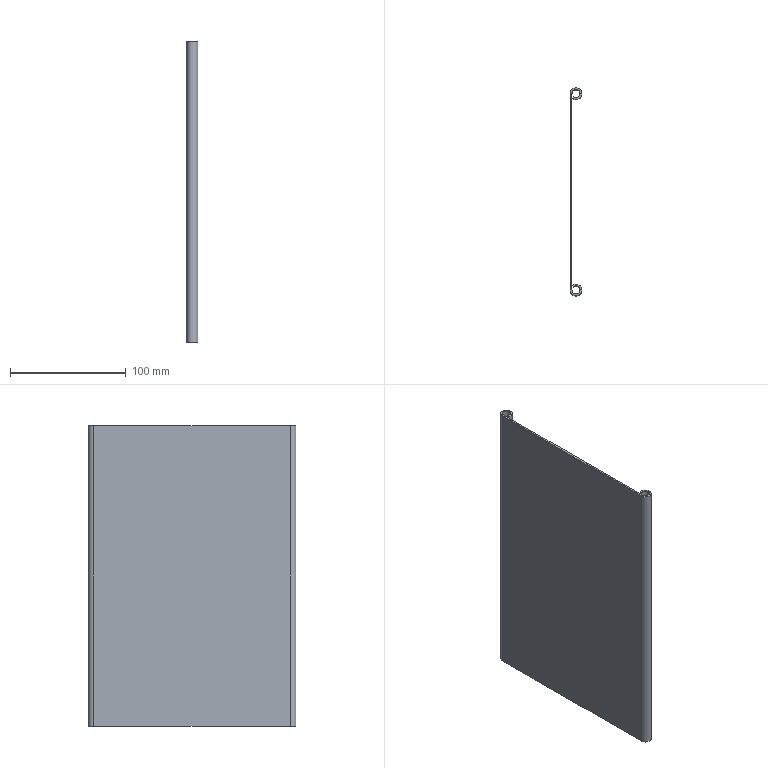Part | STEP file | Coffee machine cover door panel 001 | 1 solid | 14 faces | box 10 x 180 x 260 mm | volume 84055 mm3 | plane 10 | cylinder 4 | commonest cylinder face diameters 7 x2 10 x2
STEP:
#1=CARTESIAN_POINT('',(0.,0.,0.));
#2=DIRECTION('',(0.,0.,1.));
#3=DIRECTION('',(1.,0.,0.));
#4=AXIS2_PLACEMENT_3D('',#1,#2,#3);
#5=CARTESIAN_POINT('',(-3.5,0.,130.));
#6=VERTEX_POINT('',#5);
#7=CARTESIAN_POINT('',(-5.,0.,130.));
#8=VERTEX_POINT('',#7);
#9=CARTESIAN_POINT('',(-3.5,0.,130.));
#10=DIRECTION('',(-1.,0.,0.));
#11=VECTOR('',#10,1.);
#12=LINE('',#9,#11);
#13=CARTESIAN_POINT('',(-3.5,0.,130.));
#14=DIRECTION('',(0.,0.,1.));
#15=DIRECTION('',(1.,0.,0.));
#16=AXIS2_PLACEMENT_3D('',#13,#14,#15);
#17=PLANE('',#16);
#18=CARTESIAN_POINT('',(0.,0.));
#19=DIRECTION('',(-1.,0.));
#20=VECTOR('',#19,1.);
#21=LINE('',#18,#20);
#22=(GEOMETRIC_REPRESENTATION_CONTEXT(2)PARAMETRIC_REPRESENTATION_CONTEXT()REPRESENTATION_CONTEXT('',''));
#23=DEFINITIONAL_REPRESENTATION('',(#21),#22);
#24=PCURVE('',#17,#23);
#25=CARTESIAN_POINT('',(0.,-170.,130.));
#26=DIRECTION('',(0.,0.,1.));
#27=DIRECTION('',(1.,0.,0.));
#28=AXIS2_PLACEMENT_3D('',#25,#26,#27);
#29=PLANE('',#28);
#30=CARTESIAN_POINT('',(-3.5,170.));
#31=DIRECTION('',(-1.,0.));
#32=VECTOR('',#31,1.);
#33=LINE('',#30,#32);
#34=(GEOMETRIC_REPRESENTATION_CONTEXT(2)PARAMETRIC_REPRESENTATION_CONTEXT()REPRESENTATION_CONTEXT('',''));
#35=DEFINITIONAL_REPRESENTATION('',(#33),#34);
#36=PCURVE('',#29,#35);
#37=SURFACE_CURVE('',#12,(#24,#36),.PCURVE_S1.);
#38=EDGE_CURVE('',#6,#8,#37,.T.);
#39=ORIENTED_EDGE('',*,*,#38,.F.);
#40=CARTESIAN_POINT('',(-2.1,-2.8,130.));
#41=VERTEX_POINT('',#40);
#42=CARTESIAN_POINT('',(0.,0.,130.));
#43=DIRECTION('',(0.,0.,1.));
#44=DIRECTION('',(1.,0.,0.));
#45=AXIS2_PLACEMENT_3D('',#42,#43,#44);
#46=CIRCLE('',#45,3.5);
#47=CARTESIAN_POINT('',(3.5,0.));
#48=DIRECTION('',(1.,0.));
#49=AXIS2_PLACEMENT_2D('',#47,#48);
#50=CIRCLE('',#49,3.5);
#51=(GEOMETRIC_REPRESENTATION_CONTEXT(2)PARAMETRIC_REPRESENTATION_CONTEXT()REPRESENTATION_CONTEXT('',''));
#52=DEFINITIONAL_REPRESENTATION('',(#50),#51);
#53=PCURVE('',#17,#52);
#54=CARTESIAN_POINT('',(0.,0.,130.));
#55=DIRECTION('',(0.,0.,-1.));
#56=DIRECTION('',(-1.,0.,0.));
#57=AXIS2_PLACEMENT_3D('',#54,#55,#56);
#58=CYLINDRICAL_SURFACE('',#57,3.5);
#59=CARTESIAN_POINT('',(9.425,0.));
#60=DIRECTION('',(-1.,0.));
#61=VECTOR('',#60,1.);
#62=LINE('',#59,#61);
#63=(GEOMETRIC_REPRESENTATION_CONTEXT(2)PARAMETRIC_REPRESENTATION_CONTEXT()REPRESENTATION_CONTEXT('',''));
#64=DEFINITIONAL_REPRESENTATION('',(#62),#63);
#65=PCURVE('',#58,#64);
#66=SURFACE_CURVE('',#46,(#53,#65),.PCURVE_S1.);
#67=EDGE_CURVE('',#41,#6,#66,.T.);
#68=ORIENTED_EDGE('',*,*,#67,.F.);
#69=CARTESIAN_POINT('',(-3.,-4.,130.));
#70=VERTEX_POINT('',#69);
#71=CARTESIAN_POINT('',(-3.,-4.,130.));
#72=DIRECTION('',(0.6,0.8,0.));
#73=VECTOR('',#72,1.);
#74=LINE('',#71,#73);
#75=CARTESIAN_POINT('',(0.5,-4.));
#76=DIRECTION('',(0.6,0.8));
#77=VECTOR('',#76,1.);
#78=LINE('',#75,#77);
#79=(GEOMETRIC_REPRESENTATION_CONTEXT(2)PARAMETRIC_REPRESENTATION_CONTEXT()REPRESENTATION_CONTEXT('',''));
#80=DEFINITIONAL_REPRESENTATION('',(#78),#79);
#81=PCURVE('',#17,#80);
#82=CARTESIAN_POINT('',(-3.,-4.,130.));
#83=DIRECTION('',(-0.8,0.6,0.));
#84=DIRECTION('',(-0.6,-0.8,0.));
#85=AXIS2_PLACEMENT_3D('',#82,#83,#84);
#86=PLANE('',#85);
#87=CARTESIAN_POINT('',(0.,0.));
#88=DIRECTION('',(-1.,0.));
#89=VECTOR('',#88,1.);
#90=LINE('',#87,#89);
#91=(GEOMETRIC_REPRESENTATION_CONTEXT(2)PARAMETRIC_REPRESENTATION_CONTEXT()REPRESENTATION_CONTEXT('',''));
#92=DEFINITIONAL_REPRESENTATION('',(#90),#91);
#93=PCURVE('',#86,#92);
#94=SURFACE_CURVE('',#74,(#81,#93),.PCURVE_S1.);
#95=EDGE_CURVE('',#70,#41,#94,.T.);
#96=ORIENTED_EDGE('',*,*,#95,.F.);
#97=CARTESIAN_POINT('',(0.,0.,130.));
#98=DIRECTION('',(0.,0.,1.));
#99=DIRECTION('',(1.,0.,0.));
#100=AXIS2_PLACEMENT_3D('',#97,#98,#99);
#101=CIRCLE('',#100,5.);
#102=CARTESIAN_POINT('',(3.5,0.));
#103=DIRECTION('',(1.,0.));
#104=AXIS2_PLACEMENT_2D('',#102,#103);
#105=CIRCLE('',#104,5.);
#106=(GEOMETRIC_REPRESENTATION_CONTEXT(2)PARAMETRIC_REPRESENTATION_CONTEXT()REPRESENTATION_CONTEXT('',''));
#107=DEFINITIONAL_REPRESENTATION('',(#105),#106);
#108=PCURVE('',#17,#107);
#109=CARTESIAN_POINT('',(0.,0.,130.));
#110=DIRECTION('',(0.,0.,-1.));
#111=DIRECTION('',(-1.,0.,0.));
#112=AXIS2_PLACEMENT_3D('',#109,#110,#111);
#113=CYLINDRICAL_SURFACE('',#112,5.);
#114=CARTESIAN_POINT('',(9.425,0.));
#115=DIRECTION('',(-1.,0.));
#116=VECTOR('',#115,1.);
#117=LINE('',#114,#116);
#118=(GEOMETRIC_REPRESENTATION_CONTEXT(2)PARAMETRIC_REPRESENTATION_CONTEXT()REPRESENTATION_CONTEXT('',''));
#119=DEFINITIONAL_REPRESENTATION('',(#117),#118);
#120=PCURVE('',#113,#119);
#121=SURFACE_CURVE('',#101,(#108,#120),.PCURVE_S1.);
#122=EDGE_CURVE('',#70,#8,#121,.T.);
#123=ORIENTED_EDGE('',*,*,#122,.T.);
#124=EDGE_LOOP('',(#39,#68,#96,#123));
#125=FACE_BOUND('',#124,.T.);
#126=ADVANCED_FACE('',(#125),#17,.T.);
#127=CARTESIAN_POINT('',(-5.,0.,-130.));
#128=VERTEX_POINT('',#127);
#129=CARTESIAN_POINT('',(-3.5,0.,-130.));
#130=VERTEX_POINT('',#129);
#131=CARTESIAN_POINT('',(-5.,0.,-130.));
#132=DIRECTION('',(1.,0.,0.));
#133=VECTOR('',#132,1.);
#134=LINE('',#131,#133);
#135=CARTESIAN_POINT('',(-5.,0.,-130.));
#136=DIRECTION('',(0.,0.,-1.));
#137=DIRECTION('',(-1.,0.,0.));
#138=AXIS2_PLACEMENT_3D('',#135,#136,#137);
#139=PLANE('',#138);
#140=CARTESIAN_POINT('',(0.,0.));
#141=DIRECTION('',(-1.,0.));
#142=VECTOR('',#141,1.);
#143=LINE('',#140,#142);
#144=(GEOMETRIC_REPRESENTATION_CONTEXT(2)PARAMETRIC_REPRESENTATION_CONTEXT()REPRESENTATION_CONTEXT('',''));
#145=DEFINITIONAL_REPRESENTATION('',(#143),#144);
#146=PCURVE('',#139,#145);
#147=CARTESIAN_POINT('',(0.,-170.,-130.));
#148=DIRECTION('',(0.,0.,1.));
#149=DIRECTION('',(1.,0.,0.));
#150=AXIS2_PLACEMENT_3D('',#147,#148,#149);
#151=PLANE('',#150);
#152=CARTESIAN_POINT('',(-5.,170.));
#153=DIRECTION('',(1.,0.));
#154=VECTOR('',#153,1.);
#155=LINE('',#152,#154);
#156=(GEOMETRIC_REPRESENTATION_CONTEXT(2)PARAMETRIC_REPRESENTATION_CONTEXT()REPRESENTATION_CONTEXT('',''));
#157=DEFINITIONAL_REPRESENTATION('',(#155),#156);
#158=PCURVE('',#151,#157);
#159=SURFACE_CURVE('',#134,(#146,#158),.PCURVE_S1.);
#160=EDGE_CURVE('',#128,#130,#159,.T.);
#161=ORIENTED_EDGE('',*,*,#160,.F.);
#162=CARTESIAN_POINT('',(-3.,-4.,-130.));
#163=VERTEX_POINT('',#162);
#164=CARTESIAN_POINT('',(0.,0.,-130.));
#165=DIRECTION('',(0.,0.,1.));
#166=DIRECTION('',(1.,0.,0.));
#167=AXIS2_PLACEMENT_3D('',#164,#165,#166);
#168=CIRCLE('',#167,5.);
#169=CARTESIAN_POINT('',(-10.,0.));
#170=CARTESIAN_POINT('',(-10.,8.66));
#171=CARTESIAN_POINT('',(-2.5,4.33));
#172=CARTESIAN_POINT('',(5.,0.));
#173=CARTESIAN_POINT('',(-2.5,-4.33));
#174=CARTESIAN_POINT('',(-10.,-8.66));
#175=CARTESIAN_POINT('',(-10.,0.));
#176=(BOUNDED_CURVE()B_SPLINE_CURVE(2,(#169,#170,#171,#172,#173,#174,#175),.UNSPECIFIED.,.T.,.F.)B_SPLINE_CURVE_WITH_KNOTS((1,2,2,2,2,1),(-2.094,0.,2.094,4.189,6.283,8.378),.UNSPECIFIED.)CURVE()GEOMETRIC_REPRESENTATION_ITEM()RATIONAL_B_SPLINE_CURVE((1.,0.5,1.,0.5,1.,0.5,1.))REPRESENTATION_ITEM(''));
#177=(GEOMETRIC_REPRESENTATION_CONTEXT(2)PARAMETRIC_REPRESENTATION_CONTEXT()REPRESENTATION_CONTEXT('',''));
#178=DEFINITIONAL_REPRESENTATION('',(#176),#177);
#179=PCURVE('',#139,#178);
#180=CARTESIAN_POINT('',(9.425,260.));
#181=DIRECTION('',(-1.,0.));
#182=VECTOR('',#181,1.);
#183=LINE('',#180,#182);
#184=(GEOMETRIC_REPRESENTATION_CONTEXT(2)PARAMETRIC_REPRESENTATION_CONTEXT()REPRESENTATION_CONTEXT('',''));
#185=DEFINITIONAL_REPRESENTATION('',(#183),#184);
#186=PCURVE('',#113,#185);
#187=SURFACE_CURVE('',#168,(#179,#186),.PCURVE_S1.);
#188=EDGE_CURVE('',#163,#128,#187,.T.);
#189=ORIENTED_EDGE('',*,*,#188,.F.);
#190=CARTESIAN_POINT('',(-2.1,-2.8,-130.));
#191=VERTEX_POINT('',#190);
#192=CARTESIAN_POINT('',(-3.,-4.,-130.));
#193=DIRECTION('',(0.6,0.8,0.));
#194=VECTOR('',#193,1.);
#195=LINE('',#192,#194);
#196=CARTESIAN_POINT('',(-2.,-4.));
#197=DIRECTION('',(-0.6,0.8));
#198=VECTOR('',#197,1.);
#199=LINE('',#196,#198);
#200=(GEOMETRIC_REPRESENTATION_CONTEXT(2)PARAMETRIC_REPRESENTATION_CONTEXT()REPRESENTATION_CONTEXT('',''));
#201=DEFINITIONAL_REPRESENTATION('',(#199),#200);
#202=PCURVE('',#139,#201);
#203=CARTESIAN_POINT('',(0.,-260.));
#204=DIRECTION('',(-1.,0.));
#205=VECTOR('',#204,1.);
#206=LINE('',#203,#205);
#207=(GEOMETRIC_REPRESENTATION_CONTEXT(2)PARAMETRIC_REPRESENTATION_CONTEXT()REPRESENTATION_CONTEXT('',''));
#208=DEFINITIONAL_REPRESENTATION('',(#206),#207);
#209=PCURVE('',#86,#208);
#210=SURFACE_CURVE('',#195,(#202,#209),.PCURVE_S1.);
#211=EDGE_CURVE('',#163,#191,#210,.T.);
#212=ORIENTED_EDGE('',*,*,#211,.T.);
#213=CARTESIAN_POINT('',(0.,0.,-130.));
#214=DIRECTION('',(0.,0.,1.));
#215=DIRECTION('',(1.,0.,0.));
#216=AXIS2_PLACEMENT_3D('',#213,#214,#215);
#217=CIRCLE('',#216,3.5);
#218=CARTESIAN_POINT('',(-8.5,0.));
#219=CARTESIAN_POINT('',(-8.5,6.062));
#220=CARTESIAN_POINT('',(-3.25,3.031));
#221=CARTESIAN_POINT('',(2.,0.));
#222=CARTESIAN_POINT('',(-3.25,-3.031));
#223=CARTESIAN_POINT('',(-8.5,-6.062));
#224=CARTESIAN_POINT('',(-8.5,0.));
#225=(BOUNDED_CURVE()B_SPLINE_CURVE(2,(#218,#219,#220,#221,#222,#223,#224),.UNSPECIFIED.,.T.,.F.)B_SPLINE_CURVE_WITH_KNOTS((1,2,2,2,2,1),(-2.094,0.,2.094,4.189,6.283,8.378),.UNSPECIFIED.)CURVE()GEOMETRIC_REPRESENTATION_ITEM()RATIONAL_B_SPLINE_CURVE((1.,0.5,1.,0.5,1.,0.5,1.))REPRESENTATION_ITEM(''));
#226=(GEOMETRIC_REPRESENTATION_CONTEXT(2)PARAMETRIC_REPRESENTATION_CONTEXT()REPRESENTATION_CONTEXT('',''));
#227=DEFINITIONAL_REPRESENTATION('',(#225),#226);
#228=PCURVE('',#139,#227);
#229=CARTESIAN_POINT('',(9.425,260.));
#230=DIRECTION('',(-1.,0.));
#231=VECTOR('',#230,1.);
#232=LINE('',#229,#231);
#233=(GEOMETRIC_REPRESENTATION_CONTEXT(2)PARAMETRIC_REPRESENTATION_CONTEXT()REPRESENTATION_CONTEXT('',''));
#234=DEFINITIONAL_REPRESENTATION('',(#232),#233);
#235=PCURVE('',#58,#234);
#236=SURFACE_CURVE('',#217,(#228,#235),.PCURVE_S1.);
#237=EDGE_CURVE('',#191,#130,#236,.T.);
#238=ORIENTED_EDGE('',*,*,#237,.T.);
#239=EDGE_LOOP('',(#161,#189,#212,#238));
#240=FACE_BOUND('',#239,.T.);
#241=ADVANCED_FACE('',(#240),#139,.T.);
#242=CARTESIAN_POINT('',(-5.,-170.,130.));
#243=VERTEX_POINT('',#242);
#244=CARTESIAN_POINT('',(-3.5,-170.,130.));
#245=VERTEX_POINT('',#244);
#246=CARTESIAN_POINT('',(-5.,-170.,130.));
#247=DIRECTION('',(1.,0.,0.));
#248=VECTOR('',#247,1.);
#249=LINE('',#246,#248);
#250=CARTESIAN_POINT('',(-5.,-170.,130.));
#251=DIRECTION('',(0.,0.,1.));
#252=DIRECTION('',(1.,0.,0.));
#253=AXIS2_PLACEMENT_3D('',#250,#251,#252);
#254=PLANE('',#253);
#255=CARTESIAN_POINT('',(0.,0.));
#256=DIRECTION('',(1.,0.));
#257=VECTOR('',#256,1.);
#258=LINE('',#255,#257);
#259=(GEOMETRIC_REPRESENTATION_CONTEXT(2)PARAMETRIC_REPRESENTATION_CONTEXT()REPRESENTATION_CONTEXT('',''));
#260=DEFINITIONAL_REPRESENTATION('',(#258),#259);
#261=PCURVE('',#254,#260);
#262=CARTESIAN_POINT('',(-5.,0.));
#263=DIRECTION('',(1.,0.));
#264=VECTOR('',#263,1.);
#265=LINE('',#262,#264);
#266=(GEOMETRIC_REPRESENTATION_CONTEXT(2)PARAMETRIC_REPRESENTATION_CONTEXT()REPRESENTATION_CONTEXT('',''));
#267=DEFINITIONAL_REPRESENTATION('',(#265),#266);
#268=PCURVE('',#29,#267);
#269=SURFACE_CURVE('',#249,(#261,#268),.PCURVE_S1.);
#270=EDGE_CURVE('',#243,#245,#269,.T.);
#271=ORIENTED_EDGE('',*,*,#270,.F.);
#272=CARTESIAN_POINT('',(-3.,-166.,130.));
#273=VERTEX_POINT('',#272);
#274=CARTESIAN_POINT('',(0.,-170.,130.));
#275=DIRECTION('',(0.,0.,1.));
#276=DIRECTION('',(1.,0.,0.));
#277=AXIS2_PLACEMENT_3D('',#274,#275,#276);
#278=CIRCLE('',#277,5.);
#279=CARTESIAN_POINT('',(5.,0.));
#280=DIRECTION('',(1.,0.));
#281=AXIS2_PLACEMENT_2D('',#279,#280);
#282=CIRCLE('',#281,5.);
#283=(GEOMETRIC_REPRESENTATION_CONTEXT(2)PARAMETRIC_REPRESENTATION_CONTEXT()REPRESENTATION_CONTEXT('',''));
#284=DEFINITIONAL_REPRESENTATION('',(#282),#283);
#285=PCURVE('',#254,#284);
#286=CARTESIAN_POINT('',(0.,-170.,130.));
#287=DIRECTION('',(0.,0.,-1.));
#288=DIRECTION('',(-1.,0.,0.));
#289=AXIS2_PLACEMENT_3D('',#286,#287,#288);
#290=CYLINDRICAL_SURFACE('',#289,5.);
#291=CARTESIAN_POINT('',(9.425,0.));
#292=DIRECTION('',(-1.,0.));
#293=VECTOR('',#292,1.);
#294=LINE('',#291,#293);
#295=(GEOMETRIC_REPRESENTATION_CONTEXT(2)PARAMETRIC_REPRESENTATION_CONTEXT()REPRESENTATION_CONTEXT('',''));
#296=DEFINITIONAL_REPRESENTATION('',(#294),#295);
#297=PCURVE('',#290,#296);
#298=SURFACE_CURVE('',#278,(#285,#297),.PCURVE_S1.);
#299=EDGE_CURVE('',#243,#273,#298,.T.);
#300=ORIENTED_EDGE('',*,*,#299,.T.);
#301=CARTESIAN_POINT('',(-2.1,-167.2,130.));
#302=VERTEX_POINT('',#301);
#303=CARTESIAN_POINT('',(-2.1,-167.2,130.));
#304=DIRECTION('',(-0.6,0.8,0.));
#305=VECTOR('',#304,1.);
#306=LINE('',#303,#305);
#307=CARTESIAN_POINT('',(2.9,2.8));
#308=DIRECTION('',(-0.6,0.8));
#309=VECTOR('',#308,1.);
#310=LINE('',#307,#309);
#311=(GEOMETRIC_REPRESENTATION_CONTEXT(2)PARAMETRIC_REPRESENTATION_CONTEXT()REPRESENTATION_CONTEXT('',''));
#312=DEFINITIONAL_REPRESENTATION('',(#310),#311);
#313=PCURVE('',#254,#312);
#314=CARTESIAN_POINT('',(-2.1,-167.2,130.));
#315=DIRECTION('',(-0.8,-0.6,0.));
#316=DIRECTION('',(0.6,-0.8,0.));
#317=AXIS2_PLACEMENT_3D('',#314,#315,#316);
#318=PLANE('',#317);
#319=CARTESIAN_POINT('',(0.,0.));
#320=DIRECTION('',(-1.,0.));
#321=VECTOR('',#320,1.);
#322=LINE('',#319,#321);
#323=(GEOMETRIC_REPRESENTATION_CONTEXT(2)PARAMETRIC_REPRESENTATION_CONTEXT()REPRESENTATION_CONTEXT('',''));
#324=DEFINITIONAL_REPRESENTATION('',(#322),#323);
#325=PCURVE('',#318,#324);
#326=SURFACE_CURVE('',#306,(#313,#325),.PCURVE_S1.);
#327=EDGE_CURVE('',#302,#273,#326,.T.);
#328=ORIENTED_EDGE('',*,*,#327,.F.);
#329=CARTESIAN_POINT('',(0.,-170.,130.));
#330=DIRECTION('',(0.,0.,1.));
#331=DIRECTION('',(1.,0.,0.));
#332=AXIS2_PLACEMENT_3D('',#329,#330,#331);
#333=CIRCLE('',#332,3.5);
#334=CARTESIAN_POINT('',(5.,0.));
#335=DIRECTION('',(1.,0.));
#336=AXIS2_PLACEMENT_2D('',#334,#335);
#337=CIRCLE('',#336,3.5);
#338=(GEOMETRIC_REPRESENTATION_CONTEXT(2)PARAMETRIC_REPRESENTATION_CONTEXT()REPRESENTATION_CONTEXT('',''));
#339=DEFINITIONAL_REPRESENTATION('',(#337),#338);
#340=PCURVE('',#254,#339);
#341=CARTESIAN_POINT('',(0.,-170.,130.));
#342=DIRECTION('',(0.,0.,-1.));
#343=DIRECTION('',(-1.,0.,0.));
#344=AXIS2_PLACEMENT_3D('',#341,#342,#343);
#345=CYLINDRICAL_SURFACE('',#344,3.5);
#346=CARTESIAN_POINT('',(9.425,0.));
#347=DIRECTION('',(-1.,0.));
#348=VECTOR('',#347,1.);
#349=LINE('',#346,#348);
#350=(GEOMETRIC_REPRESENTATION_CONTEXT(2)PARAMETRIC_REPRESENTATION_CONTEXT()REPRESENTATION_CONTEXT('',''));
#351=DEFINITIONAL_REPRESENTATION('',(#349),#350);
#352=PCURVE('',#345,#351);
#353=SURFACE_CURVE('',#333,(#340,#352),.PCURVE_S1.);
#354=EDGE_CURVE('',#245,#302,#353,.T.);
#355=ORIENTED_EDGE('',*,*,#354,.F.);
#356=EDGE_LOOP('',(#271,#300,#328,#355));
#357=FACE_BOUND('',#356,.T.);
#358=ADVANCED_FACE('',(#357),#254,.T.);
#359=CARTESIAN_POINT('',(-3.5,-170.,-130.));
#360=VERTEX_POINT('',#359);
#361=CARTESIAN_POINT('',(-5.,-170.,-130.));
#362=VERTEX_POINT('',#361);
#363=CARTESIAN_POINT('',(-3.5,-170.,-130.));
#364=DIRECTION('',(-1.,0.,0.));
#365=VECTOR('',#364,1.);
#366=LINE('',#363,#365);
#367=CARTESIAN_POINT('',(-3.5,-170.,-130.));
#368=DIRECTION('',(0.,0.,-1.));
#369=DIRECTION('',(-1.,0.,0.));
#370=AXIS2_PLACEMENT_3D('',#367,#368,#369);
#371=PLANE('',#370);
#372=CARTESIAN_POINT('',(0.,0.));
#373=DIRECTION('',(1.,0.));
#374=VECTOR('',#373,1.);
#375=LINE('',#372,#374);
#376=(GEOMETRIC_REPRESENTATION_CONTEXT(2)PARAMETRIC_REPRESENTATION_CONTEXT()REPRESENTATION_CONTEXT('',''));
#377=DEFINITIONAL_REPRESENTATION('',(#375),#376);
#378=PCURVE('',#371,#377);
#379=CARTESIAN_POINT('',(-3.5,0.));
#380=DIRECTION('',(-1.,0.));
#381=VECTOR('',#380,1.);
#382=LINE('',#379,#381);
#383=(GEOMETRIC_REPRESENTATION_CONTEXT(2)PARAMETRIC_REPRESENTATION_CONTEXT()REPRESENTATION_CONTEXT('',''));
#384=DEFINITIONAL_REPRESENTATION('',(#382),#383);
#385=PCURVE('',#151,#384);
#386=SURFACE_CURVE('',#366,(#378,#385),.PCURVE_S1.);
#387=EDGE_CURVE('',#360,#362,#386,.T.);
#388=ORIENTED_EDGE('',*,*,#387,.F.);
#389=CARTESIAN_POINT('',(-2.1,-167.2,-130.));
#390=VERTEX_POINT('',#389);
#391=CARTESIAN_POINT('',(0.,-170.,-130.));
#392=DIRECTION('',(0.,0.,1.));
#393=DIRECTION('',(1.,0.,0.));
#394=AXIS2_PLACEMENT_3D('',#391,#392,#393);
#395=CIRCLE('',#394,3.5);
#396=CARTESIAN_POINT('',(-7.,0.));
#397=CARTESIAN_POINT('',(-7.,6.062));
#398=CARTESIAN_POINT('',(-1.75,3.031));
#399=CARTESIAN_POINT('',(3.5,0.));
#400=CARTESIAN_POINT('',(-1.75,-3.031));
#401=CARTESIAN_POINT('',(-7.,-6.062));
#402=CARTESIAN_POINT('',(-7.,0.));
#403=(BOUNDED_CURVE()B_SPLINE_CURVE(2,(#396,#397,#398,#399,#400,#401,#402),.UNSPECIFIED.,.T.,.F.)B_SPLINE_CURVE_WITH_KNOTS((1,2,2,2,2,1),(-2.094,0.,2.094,4.189,6.283,8.378),.UNSPECIFIED.)CURVE()GEOMETRIC_REPRESENTATION_ITEM()RATIONAL_B_SPLINE_CURVE((1.,0.5,1.,0.5,1.,0.5,1.))REPRESENTATION_ITEM(''));
#404=(GEOMETRIC_REPRESENTATION_CONTEXT(2)PARAMETRIC_REPRESENTATION_CONTEXT()REPRESENTATION_CONTEXT('',''));
#405=DEFINITIONAL_REPRESENTATION('',(#403),#404);
#406=PCURVE('',#371,#405);
#407=CARTESIAN_POINT('',(9.425,260.));
#408=DIRECTION('',(-1.,0.));
#409=VECTOR('',#408,1.);
#410=LINE('',#407,#409);
#411=(GEOMETRIC_REPRESENTATION_CONTEXT(2)PARAMETRIC_REPRESENTATION_CONTEXT()REPRESENTATION_CONTEXT('',''));
#412=DEFINITIONAL_REPRESENTATION('',(#410),#411);
#413=PCURVE('',#345,#412);
#414=SURFACE_CURVE('',#395,(#406,#413),.PCURVE_S1.);
#415=EDGE_CURVE('',#360,#390,#414,.T.);
#416=ORIENTED_EDGE('',*,*,#415,.T.);
#417=CARTESIAN_POINT('',(-3.,-166.,-130.));
#418=VERTEX_POINT('',#417);
#419=CARTESIAN_POINT('',(-2.1,-167.2,-130.));
#420=DIRECTION('',(-0.6,0.8,0.));
#421=VECTOR('',#420,1.);
#422=LINE('',#419,#421);
#423=CARTESIAN_POINT('',(-1.4,2.8));
#424=DIRECTION('',(0.6,0.8));
#425=VECTOR('',#424,1.);
#426=LINE('',#423,#425);
#427=(GEOMETRIC_REPRESENTATION_CONTEXT(2)PARAMETRIC_REPRESENTATION_CONTEXT()REPRESENTATION_CONTEXT('',''));
#428=DEFINITIONAL_REPRESENTATION('',(#426),#427);
#429=PCURVE('',#371,#428);
#430=CARTESIAN_POINT('',(0.,-260.));
#431=DIRECTION('',(-1.,0.));
#432=VECTOR('',#431,1.);
#433=LINE('',#430,#432);
#434=(GEOMETRIC_REPRESENTATION_CONTEXT(2)PARAMETRIC_REPRESENTATION_CONTEXT()REPRESENTATION_CONTEXT('',''));
#435=DEFINITIONAL_REPRESENTATION('',(#433),#434);
#436=PCURVE('',#318,#435);
#437=SURFACE_CURVE('',#422,(#429,#436),.PCURVE_S1.);
#438=EDGE_CURVE('',#390,#418,#437,.T.);
#439=ORIENTED_EDGE('',*,*,#438,.T.);
#440=CARTESIAN_POINT('',(0.,-170.,-130.));
#441=DIRECTION('',(0.,0.,1.));
#442=DIRECTION('',(1.,0.,0.));
#443=AXIS2_PLACEMENT_3D('',#440,#441,#442);
#444=CIRCLE('',#443,5.);
#445=CARTESIAN_POINT('',(-8.5,0.));
#446=CARTESIAN_POINT('',(-8.5,8.66));
#447=CARTESIAN_POINT('',(-1.,4.33));
#448=CARTESIAN_POINT('',(6.5,0.));
#449=CARTESIAN_POINT('',(-1.,-4.33));
#450=CARTESIAN_POINT('',(-8.5,-8.66));
#451=CARTESIAN_POINT('',(-8.5,0.));
#452=(BOUNDED_CURVE()B_SPLINE_CURVE(2,(#445,#446,#447,#448,#449,#450,#451),.UNSPECIFIED.,.T.,.F.)B_SPLINE_CURVE_WITH_KNOTS((1,2,2,2,2,1),(-2.094,0.,2.094,4.189,6.283,8.378),.UNSPECIFIED.)CURVE()GEOMETRIC_REPRESENTATION_ITEM()RATIONAL_B_SPLINE_CURVE((1.,0.5,1.,0.5,1.,0.5,1.))REPRESENTATION_ITEM(''));
#453=(GEOMETRIC_REPRESENTATION_CONTEXT(2)PARAMETRIC_REPRESENTATION_CONTEXT()REPRESENTATION_CONTEXT('',''));
#454=DEFINITIONAL_REPRESENTATION('',(#452),#453);
#455=PCURVE('',#371,#454);
#456=CARTESIAN_POINT('',(9.425,260.));
#457=DIRECTION('',(-1.,0.));
#458=VECTOR('',#457,1.);
#459=LINE('',#456,#458);
#460=(GEOMETRIC_REPRESENTATION_CONTEXT(2)PARAMETRIC_REPRESENTATION_CONTEXT()REPRESENTATION_CONTEXT('',''));
#461=DEFINITIONAL_REPRESENTATION('',(#459),#460);
#462=PCURVE('',#290,#461);
#463=SURFACE_CURVE('',#444,(#455,#462),.PCURVE_S1.);
#464=EDGE_CURVE('',#362,#418,#463,.T.);
#465=ORIENTED_EDGE('',*,*,#464,.F.);
#466=EDGE_LOOP('',(#388,#416,#439,#465));
#467=FACE_BOUND('',#466,.T.);
#468=ADVANCED_FACE('',(#467),#371,.T.);
#469=ORIENTED_EDGE('',*,*,#464,.T.);
#470=CARTESIAN_POINT('',(-3.,-166.,130.));
#471=DIRECTION('',(0.,0.,-1.));
#472=VECTOR('',#471,1.);
#473=LINE('',#470,#472);
#474=CARTESIAN_POINT('',(0.9273,0.));
#475=DIRECTION('',(0.,1.));
#476=VECTOR('',#475,1.);
#477=LINE('',#474,#476);
#478=(GEOMETRIC_REPRESENTATION_CONTEXT(2)PARAMETRIC_REPRESENTATION_CONTEXT()REPRESENTATION_CONTEXT('',''));
#479=DEFINITIONAL_REPRESENTATION('',(#477),#478);
#480=PCURVE('',#290,#479);
#481=CARTESIAN_POINT('',(-1.5,0.));
#482=DIRECTION('',(0.,-1.));
#483=VECTOR('',#482,1.);
#484=LINE('',#481,#483);
#485=(GEOMETRIC_REPRESENTATION_CONTEXT(2)PARAMETRIC_REPRESENTATION_CONTEXT()REPRESENTATION_CONTEXT('',''));
#486=DEFINITIONAL_REPRESENTATION('',(#484),#485);
#487=PCURVE('',#318,#486);
#488=SURFACE_CURVE('',#473,(#480,#487),.PCURVE_S1.);
#489=EDGE_CURVE('',#273,#418,#488,.T.);
#490=ORIENTED_EDGE('',*,*,#489,.F.);
#491=ORIENTED_EDGE('',*,*,#299,.F.);
#492=CARTESIAN_POINT('',(-5.,-170.,130.));
#493=DIRECTION('',(0.,0.,-1.));
#494=VECTOR('',#493,1.);
#495=LINE('',#492,#494);
#496=CARTESIAN_POINT('',(6.283,0.));
#497=DIRECTION('',(0.,1.));
#498=VECTOR('',#497,1.);
#499=LINE('',#496,#498);
#500=(GEOMETRIC_REPRESENTATION_CONTEXT(2)PARAMETRIC_REPRESENTATION_CONTEXT()REPRESENTATION_CONTEXT('',''));
#501=DEFINITIONAL_REPRESENTATION('',(#499),#500);
#502=PCURVE('',#290,#501);
#503=CARTESIAN_POINT('',(-5.,0.,130.));
#504=DIRECTION('',(1.,0.,0.));
#505=DIRECTION('',(0.,1.,0.));
#506=AXIS2_PLACEMENT_3D('',#503,#504,#505);
#507=PLANE('',#506);
#508=CARTESIAN_POINT('',(-170.,0.));
#509=DIRECTION('',(0.,-1.));
#510=VECTOR('',#509,1.);
#511=LINE('',#508,#510);
#512=(GEOMETRIC_REPRESENTATION_CONTEXT(2)PARAMETRIC_REPRESENTATION_CONTEXT()REPRESENTATION_CONTEXT('',''));
#513=DEFINITIONAL_REPRESENTATION('',(#511),#512);
#514=PCURVE('',#507,#513);
#515=SURFACE_CURVE('',#495,(#502,#514),.PCURVE_S1.);
#516=EDGE_CURVE('',#243,#362,#515,.T.);
#517=ORIENTED_EDGE('',*,*,#516,.T.);
#518=EDGE_LOOP('',(#469,#490,#491,#517));
#519=FACE_BOUND('',#518,.T.);
#520=ADVANCED_FACE('',(#519),#290,.T.);
#521=ORIENTED_EDGE('',*,*,#438,.F.);
#522=CARTESIAN_POINT('',(-2.1,-167.2,130.));
#523=DIRECTION('',(0.,0.,-1.));
#524=VECTOR('',#523,1.);
#525=LINE('',#522,#524);
#526=CARTESIAN_POINT('',(0.,0.));
#527=DIRECTION('',(0.,-1.));
#528=VECTOR('',#527,1.);
#529=LINE('',#526,#528);
#530=(GEOMETRIC_REPRESENTATION_CONTEXT(2)PARAMETRIC_REPRESENTATION_CONTEXT()REPRESENTATION_CONTEXT('',''));
#531=DEFINITIONAL_REPRESENTATION('',(#529),#530);
#532=PCURVE('',#318,#531);
#533=CARTESIAN_POINT('',(0.9273,0.));
#534=DIRECTION('',(0.,1.));
#535=VECTOR('',#534,1.);
#536=LINE('',#533,#535);
#537=(GEOMETRIC_REPRESENTATION_CONTEXT(2)PARAMETRIC_REPRESENTATION_CONTEXT()REPRESENTATION_CONTEXT('',''));
#538=DEFINITIONAL_REPRESENTATION('',(#536),#537);
#539=PCURVE('',#345,#538);
#540=SURFACE_CURVE('',#525,(#532,#539),.PCURVE_S1.);
#541=EDGE_CURVE('',#302,#390,#540,.T.);
#542=ORIENTED_EDGE('',*,*,#541,.F.);
#543=ORIENTED_EDGE('',*,*,#327,.T.);
#544=ORIENTED_EDGE('',*,*,#489,.T.);
#545=EDGE_LOOP('',(#521,#542,#543,#544));
#546=FACE_BOUND('',#545,.T.);
#547=ADVANCED_FACE('',(#546),#318,.T.);
#548=ORIENTED_EDGE('',*,*,#541,.F.);
#549=ORIENTED_EDGE('',*,*,#354,.F.);
#550=CARTESIAN_POINT('',(-3.5,-170.,130.));
#551=DIRECTION('',(0.,0.,-1.));
#552=VECTOR('',#551,1.);
#553=LINE('',#550,#552);
#554=CARTESIAN_POINT('',(6.283,0.));
#555=DIRECTION('',(0.,1.));
#556=VECTOR('',#555,1.);
#557=LINE('',#554,#556);
#558=(GEOMETRIC_REPRESENTATION_CONTEXT(2)PARAMETRIC_REPRESENTATION_CONTEXT()REPRESENTATION_CONTEXT('',''));
#559=DEFINITIONAL_REPRESENTATION('',(#557),#558);
#560=PCURVE('',#345,#559);
#561=CARTESIAN_POINT('',(-3.5,0.,130.));
#562=DIRECTION('',(1.,0.,0.));
#563=DIRECTION('',(0.,1.,0.));
#564=AXIS2_PLACEMENT_3D('',#561,#562,#563);
#565=PLANE('',#564);
#566=CARTESIAN_POINT('',(-170.,0.));
#567=DIRECTION('',(0.,-1.));
#568=VECTOR('',#567,1.);
#569=LINE('',#566,#568);
#570=(GEOMETRIC_REPRESENTATION_CONTEXT(2)PARAMETRIC_REPRESENTATION_CONTEXT()REPRESENTATION_CONTEXT('',''));
#571=DEFINITIONAL_REPRESENTATION('',(#569),#570);
#572=PCURVE('',#565,#571);
#573=SURFACE_CURVE('',#553,(#560,#572),.PCURVE_S1.);
#574=EDGE_CURVE('',#245,#360,#573,.T.);
#575=ORIENTED_EDGE('',*,*,#574,.T.);
#576=ORIENTED_EDGE('',*,*,#415,.T.);
#577=EDGE_LOOP('',(#548,#549,#575,#576));
#578=FACE_BOUND('',#577,.F.);
#579=ADVANCED_FACE('',(#578),#345,.F.);
#580=CARTESIAN_POINT('',(-3.5,0.,-130.));
#581=DIRECTION('',(0.,-1.,0.));
#582=VECTOR('',#581,1.);
#583=LINE('',#580,#582);
#584=CARTESIAN_POINT('',(0.,-260.));
#585=DIRECTION('',(-1.,0.));
#586=VECTOR('',#585,1.);
#587=LINE('',#584,#586);
#588=(GEOMETRIC_REPRESENTATION_CONTEXT(2)PARAMETRIC_REPRESENTATION_CONTEXT()REPRESENTATION_CONTEXT('',''));
#589=DEFINITIONAL_REPRESENTATION('',(#587),#588);
#590=PCURVE('',#565,#589);
#591=CARTESIAN_POINT('',(-3.5,170.));
#592=DIRECTION('',(0.,-1.));
#593=VECTOR('',#592,1.);
#594=LINE('',#591,#593);
#595=(GEOMETRIC_REPRESENTATION_CONTEXT(2)PARAMETRIC_REPRESENTATION_CONTEXT()REPRESENTATION_CONTEXT('',''));
#596=DEFINITIONAL_REPRESENTATION('',(#594),#595);
#597=PCURVE('',#151,#596);
#598=SURFACE_CURVE('',#583,(#590,#597),.PCURVE_S1.);
#599=EDGE_CURVE('',#130,#360,#598,.T.);
#600=ORIENTED_EDGE('',*,*,#599,.F.);
#601=CARTESIAN_POINT('',(-3.5,0.,130.));
#602=DIRECTION('',(0.,0.,-1.));
#603=VECTOR('',#602,1.);
#604=LINE('',#601,#603);
#605=CARTESIAN_POINT('',(0.,0.));
#606=DIRECTION('',(0.,-1.));
#607=VECTOR('',#606,1.);
#608=LINE('',#605,#607);
#609=(GEOMETRIC_REPRESENTATION_CONTEXT(2)PARAMETRIC_REPRESENTATION_CONTEXT()REPRESENTATION_CONTEXT('',''));
#610=DEFINITIONAL_REPRESENTATION('',(#608),#609);
#611=PCURVE('',#565,#610);
#612=CARTESIAN_POINT('',(0.,0.));
#613=DIRECTION('',(0.,1.));
#614=VECTOR('',#613,1.);
#615=LINE('',#612,#614);
#616=(GEOMETRIC_REPRESENTATION_CONTEXT(2)PARAMETRIC_REPRESENTATION_CONTEXT()REPRESENTATION_CONTEXT('',''));
#617=DEFINITIONAL_REPRESENTATION('',(#615),#616);
#618=PCURVE('',#58,#617);
#619=SURFACE_CURVE('',#604,(#611,#618),.PCURVE_S1.);
#620=EDGE_CURVE('',#6,#130,#619,.T.);
#621=ORIENTED_EDGE('',*,*,#620,.F.);
#622=CARTESIAN_POINT('',(-3.5,0.,130.));
#623=DIRECTION('',(0.,-1.,0.));
#624=VECTOR('',#623,1.);
#625=LINE('',#622,#624);
#626=CARTESIAN_POINT('',(0.,0.));
#627=DIRECTION('',(-1.,0.));
#628=VECTOR('',#627,1.);
#629=LINE('',#626,#628);
#630=(GEOMETRIC_REPRESENTATION_CONTEXT(2)PARAMETRIC_REPRESENTATION_CONTEXT()REPRESENTATION_CONTEXT('',''));
#631=DEFINITIONAL_REPRESENTATION('',(#629),#630);
#632=PCURVE('',#565,#631);
#633=CARTESIAN_POINT('',(-3.5,170.));
#634=DIRECTION('',(0.,-1.));
#635=VECTOR('',#634,1.);
#636=LINE('',#633,#635);
#637=(GEOMETRIC_REPRESENTATION_CONTEXT(2)PARAMETRIC_REPRESENTATION_CONTEXT()REPRESENTATION_CONTEXT('',''));
#638=DEFINITIONAL_REPRESENTATION('',(#636),#637);
#639=PCURVE('',#29,#638);
#640=SURFACE_CURVE('',#625,(#632,#639),.PCURVE_S1.);
#641=EDGE_CURVE('',#6,#245,#640,.T.);
#642=ORIENTED_EDGE('',*,*,#641,.T.);
#643=ORIENTED_EDGE('',*,*,#574,.T.);
#644=EDGE_LOOP('',(#600,#621,#642,#643));
#645=FACE_BOUND('',#644,.T.);
#646=ADVANCED_FACE('',(#645),#565,.T.);
#647=ORIENTED_EDGE('',*,*,#620,.F.);
#648=ORIENTED_EDGE('',*,*,#67,.F.);
#649=CARTESIAN_POINT('',(-2.1,-2.8,130.));
#650=DIRECTION('',(0.,0.,-1.));
#651=VECTOR('',#650,1.);
#652=LINE('',#649,#651);
#653=CARTESIAN_POINT('',(5.356,0.));
#654=DIRECTION('',(0.,1.));
#655=VECTOR('',#654,1.);
#656=LINE('',#653,#655);
#657=(GEOMETRIC_REPRESENTATION_CONTEXT(2)PARAMETRIC_REPRESENTATION_CONTEXT()REPRESENTATION_CONTEXT('',''));
#658=DEFINITIONAL_REPRESENTATION('',(#656),#657);
#659=PCURVE('',#58,#658);
#660=CARTESIAN_POINT('',(-1.5,0.));
#661=DIRECTION('',(0.,-1.));
#662=VECTOR('',#661,1.);
#663=LINE('',#660,#662);
#664=(GEOMETRIC_REPRESENTATION_CONTEXT(2)PARAMETRIC_REPRESENTATION_CONTEXT()REPRESENTATION_CONTEXT('',''));
#665=DEFINITIONAL_REPRESENTATION('',(#663),#664);
#666=PCURVE('',#86,#665);
#667=SURFACE_CURVE('',#652,(#659,#666),.PCURVE_S1.);
#668=EDGE_CURVE('',#41,#191,#667,.T.);
#669=ORIENTED_EDGE('',*,*,#668,.T.);
#670=ORIENTED_EDGE('',*,*,#237,.T.);
#671=EDGE_LOOP('',(#647,#648,#669,#670));
#672=FACE_BOUND('',#671,.F.);
#673=ADVANCED_FACE('',(#672),#58,.F.);
#674=ORIENTED_EDGE('',*,*,#211,.F.);
#675=CARTESIAN_POINT('',(-3.,-4.,130.));
#676=DIRECTION('',(0.,0.,-1.));
#677=VECTOR('',#676,1.);
#678=LINE('',#675,#677);
#679=CARTESIAN_POINT('',(0.,0.));
#680=DIRECTION('',(0.,-1.));
#681=VECTOR('',#680,1.);
#682=LINE('',#679,#681);
#683=(GEOMETRIC_REPRESENTATION_CONTEXT(2)PARAMETRIC_REPRESENTATION_CONTEXT()REPRESENTATION_CONTEXT('',''));
#684=DEFINITIONAL_REPRESENTATION('',(#682),#683);
#685=PCURVE('',#86,#684);
#686=CARTESIAN_POINT('',(5.356,0.));
#687=DIRECTION('',(0.,1.));
#688=VECTOR('',#687,1.);
#689=LINE('',#686,#688);
#690=(GEOMETRIC_REPRESENTATION_CONTEXT(2)PARAMETRIC_REPRESENTATION_CONTEXT()REPRESENTATION_CONTEXT('',''));
#691=DEFINITIONAL_REPRESENTATION('',(#689),#690);
#692=PCURVE('',#113,#691);
#693=SURFACE_CURVE('',#678,(#685,#692),.PCURVE_S1.);
#694=EDGE_CURVE('',#70,#163,#693,.T.);
#695=ORIENTED_EDGE('',*,*,#694,.F.);
#696=ORIENTED_EDGE('',*,*,#95,.T.);
#697=ORIENTED_EDGE('',*,*,#668,.T.);
#698=EDGE_LOOP('',(#674,#695,#696,#697));
#699=FACE_BOUND('',#698,.T.);
#700=ADVANCED_FACE('',(#699),#86,.T.);
#701=ORIENTED_EDGE('',*,*,#188,.T.);
#702=CARTESIAN_POINT('',(-5.,0.,130.));
#703=DIRECTION('',(0.,0.,-1.));
#704=VECTOR('',#703,1.);
#705=LINE('',#702,#704);
#706=CARTESIAN_POINT('',(0.,0.));
#707=DIRECTION('',(0.,1.));
#708=VECTOR('',#707,1.);
#709=LINE('',#706,#708);
#710=(GEOMETRIC_REPRESENTATION_CONTEXT(2)PARAMETRIC_REPRESENTATION_CONTEXT()REPRESENTATION_CONTEXT('',''));
#711=DEFINITIONAL_REPRESENTATION('',(#709),#710);
#712=PCURVE('',#113,#711);
#713=CARTESIAN_POINT('',(0.,0.));
#714=DIRECTION('',(0.,-1.));
#715=VECTOR('',#714,1.);
#716=LINE('',#713,#715);
#717=(GEOMETRIC_REPRESENTATION_CONTEXT(2)PARAMETRIC_REPRESENTATION_CONTEXT()REPRESENTATION_CONTEXT('',''));
#718=DEFINITIONAL_REPRESENTATION('',(#716),#717);
#719=PCURVE('',#507,#718);
#720=SURFACE_CURVE('',#705,(#712,#719),.PCURVE_S1.);
#721=EDGE_CURVE('',#8,#128,#720,.T.);
#722=ORIENTED_EDGE('',*,*,#721,.F.);
#723=ORIENTED_EDGE('',*,*,#122,.F.);
#724=ORIENTED_EDGE('',*,*,#694,.T.);
#725=EDGE_LOOP('',(#701,#722,#723,#724));
#726=FACE_BOUND('',#725,.T.);
#727=ADVANCED_FACE('',(#726),#113,.T.);
#728=CARTESIAN_POINT('',(-5.,0.,-130.));
#729=DIRECTION('',(0.,-1.,0.));
#730=VECTOR('',#729,1.);
#731=LINE('',#728,#730);
#732=CARTESIAN_POINT('',(0.,-260.));
#733=DIRECTION('',(-1.,0.));
#734=VECTOR('',#733,1.);
#735=LINE('',#732,#734);
#736=(GEOMETRIC_REPRESENTATION_CONTEXT(2)PARAMETRIC_REPRESENTATION_CONTEXT()REPRESENTATION_CONTEXT('',''));
#737=DEFINITIONAL_REPRESENTATION('',(#735),#736);
#738=PCURVE('',#507,#737);
#739=CARTESIAN_POINT('',(-5.,170.));
#740=DIRECTION('',(0.,-1.));
#741=VECTOR('',#740,1.);
#742=LINE('',#739,#741);
#743=(GEOMETRIC_REPRESENTATION_CONTEXT(2)PARAMETRIC_REPRESENTATION_CONTEXT()REPRESENTATION_CONTEXT('',''));
#744=DEFINITIONAL_REPRESENTATION('',(#742),#743);
#745=PCURVE('',#151,#744);
#746=SURFACE_CURVE('',#731,(#738,#745),.PCURVE_S1.);
#747=EDGE_CURVE('',#128,#362,#746,.T.);
#748=ORIENTED_EDGE('',*,*,#747,.T.);
#749=ORIENTED_EDGE('',*,*,#516,.F.);
#750=CARTESIAN_POINT('',(-5.,0.,130.));
#751=DIRECTION('',(0.,-1.,0.));
#752=VECTOR('',#751,1.);
#753=LINE('',#750,#752);
#754=CARTESIAN_POINT('',(0.,0.));
#755=DIRECTION('',(-1.,0.));
#756=VECTOR('',#755,1.);
#757=LINE('',#754,#756);
#758=(GEOMETRIC_REPRESENTATION_CONTEXT(2)PARAMETRIC_REPRESENTATION_CONTEXT()REPRESENTATION_CONTEXT('',''));
#759=DEFINITIONAL_REPRESENTATION('',(#757),#758);
#760=PCURVE('',#507,#759);
#761=CARTESIAN_POINT('',(-5.,170.));
#762=DIRECTION('',(0.,-1.));
#763=VECTOR('',#762,1.);
#764=LINE('',#761,#763);
#765=(GEOMETRIC_REPRESENTATION_CONTEXT(2)PARAMETRIC_REPRESENTATION_CONTEXT()REPRESENTATION_CONTEXT('',''));
#766=DEFINITIONAL_REPRESENTATION('',(#764),#765);
#767=PCURVE('',#29,#766);
#768=SURFACE_CURVE('',#753,(#760,#767),.PCURVE_S1.);
#769=EDGE_CURVE('',#8,#243,#768,.T.);
#770=ORIENTED_EDGE('',*,*,#769,.F.);
#771=ORIENTED_EDGE('',*,*,#721,.T.);
#772=EDGE_LOOP('',(#748,#749,#770,#771));
#773=FACE_BOUND('',#772,.T.);
#774=ADVANCED_FACE('',(#773),#507,.F.);
#775=ORIENTED_EDGE('',*,*,#769,.T.);
#776=ORIENTED_EDGE('',*,*,#270,.T.);
#777=ORIENTED_EDGE('',*,*,#641,.F.);
#778=ORIENTED_EDGE('',*,*,#38,.T.);
#779=EDGE_LOOP('',(#775,#776,#777,#778));
#780=FACE_BOUND('',#779,.T.);
#781=ADVANCED_FACE('',(#780),#29,.T.);
#782=ORIENTED_EDGE('',*,*,#599,.T.);
#783=ORIENTED_EDGE('',*,*,#387,.T.);
#784=ORIENTED_EDGE('',*,*,#747,.F.);
#785=ORIENTED_EDGE('',*,*,#160,.T.);
#786=EDGE_LOOP('',(#782,#783,#784,#785));
#787=FACE_BOUND('',#786,.T.);
#788=ADVANCED_FACE('',(#787),#151,.F.);
#789=CLOSED_SHELL('',(#126,#241,#358,#468,#520,#547,#579,#646,#673,#700,#727,#774,#781,#788));
#790=MANIFOLD_SOLID_BREP('',#789);
#791=(LENGTH_UNIT()NAMED_UNIT(*)SI_UNIT(.MILLI.,.METRE.));
#792=UNCERTAINTY_MEASURE_WITH_UNIT(LENGTH_MEASURE(0.0000001),#791,'','');
#793=(NAMED_UNIT(*)PLANE_ANGLE_UNIT()SI_UNIT($,.RADIAN.));
#794=(NAMED_UNIT(*)SI_UNIT($,.STERADIAN.)SOLID_ANGLE_UNIT());
#795=(GEOMETRIC_REPRESENTATION_CONTEXT(3)GLOBAL_UNCERTAINTY_ASSIGNED_CONTEXT((#792))GLOBAL_UNIT_ASSIGNED_CONTEXT((#791,#793,#794))REPRESENTATION_CONTEXT('',''));
#796=ADVANCED_BREP_SHAPE_REPRESENTATION('',(#4,#790),#795);